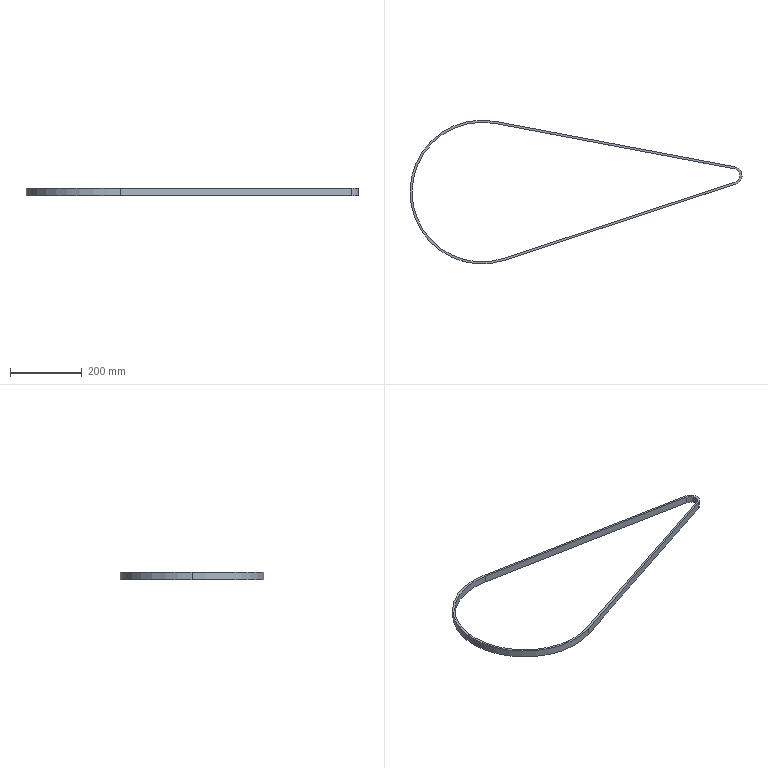Part | SolidWorks | features Sweep 1 | 1 solid | 12 faces | box 923.5 x 400 x 20 mm | volume 251339 mm3 | cylinder 6 | plane 6 | commonest cylinder face diameters 388.216 x2 400 x2 38.274 x1 50 x1
STEP:
#1=CARTESIAN_POINT('',(-778.071,-459.045,10.));
#2=VERTEX_POINT('',#1);
#3=CARTESIAN_POINT('',(-1040.663,-269.092,10.));
#4=VERTEX_POINT('',#3);
#5=CARTESIAN_POINT('',(-840.663,-269.092,10.));
#6=DIRECTION('',(0.,0.,-1.));
#7=DIRECTION('',(-1.,0.,0.));
#8=AXIS2_PLACEMENT_3D('',#5,#6,#7);
#9=CIRCLE('',#8,200.);
#10=EDGE_CURVE('',#2,#4,#9,.T.);
#11=ORIENTED_EDGE('',*,*,#10,.T.);
#12=CARTESIAN_POINT('',(-1040.663,-269.092,-10.));
#13=VERTEX_POINT('',#12);
#14=CARTESIAN_POINT('',(-1040.663,-269.092,0.));
#15=DIRECTION('',(0.,0.,-1.));
#16=VECTOR('',#15,1000.);
#17=LINE('',#14,#16);
#18=EDGE_CURVE('',#4,#13,#17,.T.);
#19=ORIENTED_EDGE('',*,*,#18,.T.);
#20=CARTESIAN_POINT('',(-778.071,-459.045,-10.));
#21=VERTEX_POINT('',#20);
#22=CARTESIAN_POINT('',(-840.663,-269.092,-10.));
#23=DIRECTION('',(0.,0.,-1.));
#24=DIRECTION('',(-1.,0.,0.));
#25=AXIS2_PLACEMENT_3D('',#22,#23,#24);
#26=CIRCLE('',#25,200.);
#27=EDGE_CURVE('',#21,#13,#26,.T.);
#28=ORIENTED_EDGE('',*,*,#27,.F.);
#29=CARTESIAN_POINT('',(-778.071,-459.045,10.));
#30=DIRECTION('',(0.,0.,1.));
#31=VECTOR('',#30,1000.);
#32=LINE('',#29,#31);
#33=EDGE_CURVE('',#21,#2,#32,.T.);
#34=ORIENTED_EDGE('',*,*,#33,.T.);
#35=EDGE_LOOP('',(#11,#19,#28,#34));
#36=FACE_OUTER_BOUND('',#35,.T.);
#37=CARTESIAN_POINT('',(-840.663,-269.092,0.));
#38=DIRECTION('',(0.,0.,-1.));
#39=DIRECTION('',(-1.,0.,0.));
#40=AXIS2_PLACEMENT_3D('',#37,#38,#39);
#41=CYLINDRICAL_SURFACE('',#40,200.);
#42=ADVANCED_FACE('',(#36),#41,.T.);
#43=CARTESIAN_POINT('',(-1034.771,-269.092,10.));
#44=VERTEX_POINT('',#43);
#45=CARTESIAN_POINT('',(-803.472,-78.58,10.));
#46=VERTEX_POINT('',#45);
#47=CARTESIAN_POINT('',(-840.663,-269.092,10.));
#48=DIRECTION('',(0.,0.,-1.));
#49=DIRECTION('',(-1.,0.,0.));
#50=AXIS2_PLACEMENT_3D('',#47,#48,#49);
#51=CIRCLE('',#50,194.108);
#52=EDGE_CURVE('',#44,#46,#51,.T.);
#53=ORIENTED_EDGE('',*,*,#52,.F.);
#54=CARTESIAN_POINT('',(-1034.771,-269.092,-10.));
#55=VERTEX_POINT('',#54);
#56=CARTESIAN_POINT('',(-1034.771,-269.092,0.));
#57=DIRECTION('',(0.,0.,-1.));
#58=VECTOR('',#57,1000.);
#59=LINE('',#56,#58);
#60=EDGE_CURVE('',#44,#55,#59,.T.);
#61=ORIENTED_EDGE('',*,*,#60,.T.);
#62=CARTESIAN_POINT('',(-803.472,-78.58,-10.));
#63=VERTEX_POINT('',#62);
#64=CARTESIAN_POINT('',(-840.663,-269.092,-10.));
#65=DIRECTION('',(0.,0.,-1.));
#66=DIRECTION('',(-1.,0.,0.));
#67=AXIS2_PLACEMENT_3D('',#64,#65,#66);
#68=CIRCLE('',#67,194.108);
#69=EDGE_CURVE('',#55,#63,#68,.T.);
#70=ORIENTED_EDGE('',*,*,#69,.T.);
#71=CARTESIAN_POINT('',(-803.472,-78.58,10.));
#72=CARTESIAN_POINT('',(-803.472,-78.58,3.333));
#73=CARTESIAN_POINT('',(-803.472,-78.58,-3.333));
#74=CARTESIAN_POINT('',(-803.472,-78.58,-10.));
#75=B_SPLINE_CURVE_WITH_KNOTS('',3,(#71,#72,#73,#74),.UNSPECIFIED.,.F.,.F.,(4,4),(0.,1.),.UNSPECIFIED.);
#76=EDGE_CURVE('',#46,#63,#75,.T.);
#77=ORIENTED_EDGE('',*,*,#76,.F.);
#78=EDGE_LOOP('',(#53,#61,#70,#77));
#79=FACE_OUTER_BOUND('',#78,.T.);
#80=CARTESIAN_POINT('',(-840.663,-269.092,0.));
#81=DIRECTION('',(0.,0.,-1.));
#82=DIRECTION('',(-1.,0.,0.));
#83=AXIS2_PLACEMENT_3D('',#80,#81,#82);
#84=CYLINDRICAL_SURFACE('',#83,194.108);
#85=ADVANCED_FACE('',(#79),#84,.F.);
#86=ORIENTED_EDGE('',*,*,#60,.F.);
#87=CARTESIAN_POINT('',(-780.976,-453.795,10.));
#88=VERTEX_POINT('',#87);
#89=CARTESIAN_POINT('',(-840.663,-269.092,10.));
#90=DIRECTION('',(0.,0.,-1.));
#91=DIRECTION('',(-1.,0.,0.));
#92=AXIS2_PLACEMENT_3D('',#89,#90,#91);
#93=CIRCLE('',#92,194.108);
#94=EDGE_CURVE('',#88,#44,#93,.T.);
#95=ORIENTED_EDGE('',*,*,#94,.F.);
#96=CARTESIAN_POINT('',(-780.976,-453.795,-10.));
#97=VERTEX_POINT('',#96);
#98=CARTESIAN_POINT('',(-780.976,-453.795,10.));
#99=DIRECTION('',(0.,0.,-1.));
#100=VECTOR('',#99,1000.);
#101=LINE('',#98,#100);
#102=EDGE_CURVE('',#88,#97,#101,.T.);
#103=ORIENTED_EDGE('',*,*,#102,.T.);
#104=CARTESIAN_POINT('',(-840.663,-269.092,-10.));
#105=DIRECTION('',(0.,0.,-1.));
#106=DIRECTION('',(-1.,0.,0.));
#107=AXIS2_PLACEMENT_3D('',#104,#105,#106);
#108=CIRCLE('',#107,194.108);
#109=EDGE_CURVE('',#97,#55,#108,.T.);
#110=ORIENTED_EDGE('',*,*,#109,.T.);
#111=EDGE_LOOP('',(#86,#95,#103,#110));
#112=FACE_OUTER_BOUND('',#111,.T.);
#113=CARTESIAN_POINT('',(-840.663,-269.092,0.));
#114=DIRECTION('',(0.,0.,-1.));
#115=DIRECTION('',(-1.,0.,0.));
#116=AXIS2_PLACEMENT_3D('',#113,#114,#115);
#117=CYLINDRICAL_SURFACE('',#116,194.108);
#118=ADVANCED_FACE('',(#112),#117,.F.);
#119=ORIENTED_EDGE('',*,*,#18,.F.);
#120=CARTESIAN_POINT('',(-803.472,-72.58,10.));
#121=VERTEX_POINT('',#120);
#122=CARTESIAN_POINT('',(-840.663,-269.092,10.));
#123=DIRECTION('',(0.,0.,-1.));
#124=DIRECTION('',(-1.,0.,0.));
#125=AXIS2_PLACEMENT_3D('',#122,#123,#124);
#126=CIRCLE('',#125,200.);
#127=EDGE_CURVE('',#4,#121,#126,.T.);
#128=ORIENTED_EDGE('',*,*,#127,.T.);
#129=CARTESIAN_POINT('',(-803.472,-72.58,-10.));
#130=VERTEX_POINT('',#129);
#131=CARTESIAN_POINT('',(-803.472,-72.58,-10.));
#132=CARTESIAN_POINT('',(-803.472,-72.58,-3.333));
#133=CARTESIAN_POINT('',(-803.472,-72.58,3.333));
#134=CARTESIAN_POINT('',(-803.472,-72.58,10.));
#135=B_SPLINE_CURVE_WITH_KNOTS('',3,(#131,#132,#133,#134),.UNSPECIFIED.,.F.,.F.,(4,4),(0.,1.),.UNSPECIFIED.);
#136=EDGE_CURVE('',#130,#121,#135,.T.);
#137=ORIENTED_EDGE('',*,*,#136,.F.);
#138=CARTESIAN_POINT('',(-840.663,-269.092,-10.));
#139=DIRECTION('',(0.,0.,-1.));
#140=DIRECTION('',(-1.,0.,0.));
#141=AXIS2_PLACEMENT_3D('',#138,#139,#140);
#142=CIRCLE('',#141,200.);
#143=EDGE_CURVE('',#13,#130,#142,.T.);
#144=ORIENTED_EDGE('',*,*,#143,.F.);
#145=EDGE_LOOP('',(#119,#128,#137,#144));
#146=FACE_OUTER_BOUND('',#145,.T.);
#147=CARTESIAN_POINT('',(-840.663,-269.092,0.));
#148=DIRECTION('',(0.,0.,-1.));
#149=DIRECTION('',(-1.,0.,0.));
#150=AXIS2_PLACEMENT_3D('',#147,#148,#149);
#151=CYLINDRICAL_SURFACE('',#150,200.);
#152=ADVANCED_FACE('',(#146),#151,.T.);
#153=CARTESIAN_POINT('',(-137.244,-241.677,10.));
#154=VERTEX_POINT('',#153);
#155=CARTESIAN_POINT('',(-137.244,-241.677,-10.));
#156=VERTEX_POINT('',#155);
#157=CARTESIAN_POINT('',(-137.244,-241.677,10.));
#158=DIRECTION('',(0.,0.,-1.));
#159=VECTOR('',#158,1000.);
#160=LINE('',#157,#159);
#161=EDGE_CURVE('',#154,#156,#160,.T.);
#162=ORIENTED_EDGE('',*,*,#161,.T.);
#163=CARTESIAN_POINT('',(-137.244,-241.677,-10.));
#164=DIRECTION('',(-0.9498,-0.313,0.));
#165=VECTOR('',#164,1000.);
#166=LINE('',#163,#165);
#167=EDGE_CURVE('',#156,#97,#166,.T.);
#168=ORIENTED_EDGE('',*,*,#167,.T.);
#169=ORIENTED_EDGE('',*,*,#102,.F.);
#170=CARTESIAN_POINT('',(-137.244,-241.677,10.));
#171=DIRECTION('',(-0.9498,-0.313,0.));
#172=VECTOR('',#171,1000.);
#173=LINE('',#170,#172);
#174=EDGE_CURVE('',#154,#88,#173,.T.);
#175=ORIENTED_EDGE('',*,*,#174,.F.);
#176=EDGE_LOOP('',(#162,#168,#169,#175));
#177=FACE_OUTER_BOUND('',#176,.T.);
#178=CARTESIAN_POINT('',(-137.244,-241.677,10.));
#179=DIRECTION('',(-0.313,0.9498,0.));
#180=DIRECTION('',(-0.9498,-0.313,0.));
#181=AXIS2_PLACEMENT_3D('',#178,#179,#180);
#182=PLANE('',#181);
#183=ADVANCED_FACE('',(#177),#182,.T.);
#184=CARTESIAN_POINT('',(-134.34,-246.927,-10.));
#185=VERTEX_POINT('',#184);
#186=CARTESIAN_POINT('',(-134.34,-246.927,10.));
#187=VERTEX_POINT('',#186);
#188=CARTESIAN_POINT('',(-134.34,-246.927,10.));
#189=DIRECTION('',(0.,0.,1.));
#190=VECTOR('',#189,1000.);
#191=LINE('',#188,#190);
#192=EDGE_CURVE('',#185,#187,#191,.T.);
#193=ORIENTED_EDGE('',*,*,#192,.T.);
#194=CARTESIAN_POINT('',(-134.34,-246.927,10.));
#195=DIRECTION('',(-0.9498,-0.313,0.));
#196=VECTOR('',#195,1000.);
#197=LINE('',#194,#196);
#198=EDGE_CURVE('',#187,#2,#197,.T.);
#199=ORIENTED_EDGE('',*,*,#198,.T.);
#200=ORIENTED_EDGE('',*,*,#33,.F.);
#201=CARTESIAN_POINT('',(-134.34,-246.927,-10.));
#202=DIRECTION('',(-0.9498,-0.313,0.));
#203=VECTOR('',#202,1000.);
#204=LINE('',#201,#203);
#205=EDGE_CURVE('',#185,#21,#204,.T.);
#206=ORIENTED_EDGE('',*,*,#205,.F.);
#207=EDGE_LOOP('',(#193,#199,#200,#206));
#208=FACE_OUTER_BOUND('',#207,.T.);
#209=CARTESIAN_POINT('',(-134.34,-246.927,10.));
#210=DIRECTION('',(0.313,-0.9498,0.));
#211=DIRECTION('',(0.9498,0.313,0.));
#212=AXIS2_PLACEMENT_3D('',#209,#210,#211);
#213=PLANE('',#212);
#214=ADVANCED_FACE('',(#208),#213,.T.);
#215=CARTESIAN_POINT('',(-137.515,-204.619,10.));
#216=VERTEX_POINT('',#215);
#217=CARTESIAN_POINT('',(-137.515,-204.619,-10.));
#218=VERTEX_POINT('',#217);
#219=CARTESIAN_POINT('',(-137.515,-204.619,10.));
#220=DIRECTION('',(0.,0.,-1.));
#221=VECTOR('',#220,1000.);
#222=LINE('',#219,#221);
#223=EDGE_CURVE('',#216,#218,#222,.T.);
#224=ORIENTED_EDGE('',*,*,#223,.T.);
#225=CARTESIAN_POINT('',(-142.164,-223.183,-10.));
#226=DIRECTION('',(0.,0.,-1.));
#227=DIRECTION('',(-1.,0.,0.));
#228=AXIS2_PLACEMENT_3D('',#225,#226,#227);
#229=CIRCLE('',#228,19.137);
#230=EDGE_CURVE('',#218,#156,#229,.T.);
#231=ORIENTED_EDGE('',*,*,#230,.T.);
#232=ORIENTED_EDGE('',*,*,#161,.F.);
#233=CARTESIAN_POINT('',(-142.164,-223.183,10.));
#234=DIRECTION('',(0.,0.,-1.));
#235=DIRECTION('',(-1.,0.,0.));
#236=AXIS2_PLACEMENT_3D('',#233,#234,#235);
#237=CIRCLE('',#236,19.137);
#238=EDGE_CURVE('',#216,#154,#237,.T.);
#239=ORIENTED_EDGE('',*,*,#238,.F.);
#240=EDGE_LOOP('',(#224,#231,#232,#239));
#241=FACE_OUTER_BOUND('',#240,.T.);
#242=CARTESIAN_POINT('',(-142.164,-223.183,0.));
#243=DIRECTION('',(0.,0.,-1.));
#244=DIRECTION('',(-1.,0.,0.));
#245=AXIS2_PLACEMENT_3D('',#242,#243,#244);
#246=CYLINDRICAL_SURFACE('',#245,19.137);
#247=ADVANCED_FACE('',(#241),#246,.F.);
#248=CARTESIAN_POINT('',(-137.515,-198.619,-10.));
#249=VERTEX_POINT('',#248);
#250=CARTESIAN_POINT('',(-137.515,-198.619,10.));
#251=VERTEX_POINT('',#250);
#252=CARTESIAN_POINT('',(-137.515,-198.619,10.));
#253=DIRECTION('',(0.,0.,1.));
#254=VECTOR('',#253,1000.);
#255=LINE('',#252,#254);
#256=EDGE_CURVE('',#249,#251,#255,.T.);
#257=ORIENTED_EDGE('',*,*,#256,.T.);
#258=CARTESIAN_POINT('',(-142.164,-223.183,10.));
#259=DIRECTION('',(0.,0.,-1.));
#260=DIRECTION('',(-1.,0.,0.));
#261=AXIS2_PLACEMENT_3D('',#258,#259,#260);
#262=CIRCLE('',#261,25.);
#263=EDGE_CURVE('',#251,#187,#262,.T.);
#264=ORIENTED_EDGE('',*,*,#263,.T.);
#265=ORIENTED_EDGE('',*,*,#192,.F.);
#266=CARTESIAN_POINT('',(-142.164,-223.183,-10.));
#267=DIRECTION('',(0.,0.,-1.));
#268=DIRECTION('',(-1.,0.,0.));
#269=AXIS2_PLACEMENT_3D('',#266,#267,#268);
#270=CIRCLE('',#269,25.);
#271=EDGE_CURVE('',#249,#185,#270,.T.);
#272=ORIENTED_EDGE('',*,*,#271,.F.);
#273=EDGE_LOOP('',(#257,#264,#265,#272));
#274=FACE_OUTER_BOUND('',#273,.T.);
#275=CARTESIAN_POINT('',(-142.164,-223.183,0.));
#276=DIRECTION('',(0.,0.,-1.));
#277=DIRECTION('',(-1.,0.,0.));
#278=AXIS2_PLACEMENT_3D('',#275,#276,#277);
#279=CYLINDRICAL_SURFACE('',#278,25.);
#280=ADVANCED_FACE('',(#274),#279,.T.);
#281=CARTESIAN_POINT('',(-137.515,-204.619,10.));
#282=DIRECTION('',(-0.9826,0.186,0.));
#283=VECTOR('',#282,1000.);
#284=LINE('',#281,#283);
#285=EDGE_CURVE('',#216,#46,#284,.T.);
#286=ORIENTED_EDGE('',*,*,#285,.F.);
#287=ORIENTED_EDGE('',*,*,#238,.T.);
#288=ORIENTED_EDGE('',*,*,#174,.T.);
#289=ORIENTED_EDGE('',*,*,#94,.T.);
#290=ORIENTED_EDGE('',*,*,#52,.T.);
#291=EDGE_LOOP('',(#286,#287,#288,#289,#290));
#292=FACE_BOUND('',#291,.T.);
#293=CARTESIAN_POINT('',(-137.515,-198.619,10.));
#294=DIRECTION('',(-0.9826,0.186,0.));
#295=VECTOR('',#294,1000.);
#296=LINE('',#293,#295);
#297=EDGE_CURVE('',#251,#121,#296,.T.);
#298=ORIENTED_EDGE('',*,*,#297,.T.);
#299=ORIENTED_EDGE('',*,*,#127,.F.);
#300=ORIENTED_EDGE('',*,*,#10,.F.);
#301=ORIENTED_EDGE('',*,*,#198,.F.);
#302=ORIENTED_EDGE('',*,*,#263,.F.);
#303=EDGE_LOOP('',(#298,#299,#300,#301,#302));
#304=FACE_OUTER_BOUND('',#303,.T.);
#305=CARTESIAN_POINT('',(-137.515,-198.619,10.));
#306=DIRECTION('',(0.,0.,-1.));
#307=DIRECTION('',(0.,1.,0.));
#308=AXIS2_PLACEMENT_3D('',#305,#306,#307);
#309=PLANE('',#308);
#310=ADVANCED_FACE('',(#292,#304),#309,.F.);
#311=ORIENTED_EDGE('',*,*,#76,.T.);
#312=CARTESIAN_POINT('',(-137.515,-204.619,-10.));
#313=DIRECTION('',(-0.9826,0.186,0.));
#314=VECTOR('',#313,1000.);
#315=LINE('',#312,#314);
#316=EDGE_CURVE('',#218,#63,#315,.T.);
#317=ORIENTED_EDGE('',*,*,#316,.F.);
#318=ORIENTED_EDGE('',*,*,#223,.F.);
#319=ORIENTED_EDGE('',*,*,#285,.T.);
#320=EDGE_LOOP('',(#311,#317,#318,#319));
#321=FACE_OUTER_BOUND('',#320,.T.);
#322=CARTESIAN_POINT('',(-137.515,-204.619,10.));
#323=DIRECTION('',(0.186,0.9826,0.));
#324=DIRECTION('',(-0.9826,0.186,0.));
#325=AXIS2_PLACEMENT_3D('',#322,#323,#324);
#326=PLANE('',#325);
#327=ADVANCED_FACE('',(#321),#326,.F.);
#328=CARTESIAN_POINT('',(-137.515,-198.619,-10.));
#329=DIRECTION('',(-0.9826,0.186,0.));
#330=VECTOR('',#329,1000.);
#331=LINE('',#328,#330);
#332=EDGE_CURVE('',#249,#130,#331,.T.);
#333=ORIENTED_EDGE('',*,*,#332,.F.);
#334=ORIENTED_EDGE('',*,*,#271,.T.);
#335=ORIENTED_EDGE('',*,*,#205,.T.);
#336=ORIENTED_EDGE('',*,*,#27,.T.);
#337=ORIENTED_EDGE('',*,*,#143,.T.);
#338=EDGE_LOOP('',(#333,#334,#335,#336,#337));
#339=FACE_OUTER_BOUND('',#338,.T.);
#340=ORIENTED_EDGE('',*,*,#316,.T.);
#341=ORIENTED_EDGE('',*,*,#69,.F.);
#342=ORIENTED_EDGE('',*,*,#109,.F.);
#343=ORIENTED_EDGE('',*,*,#167,.F.);
#344=ORIENTED_EDGE('',*,*,#230,.F.);
#345=EDGE_LOOP('',(#340,#341,#342,#343,#344));
#346=FACE_BOUND('',#345,.T.);
#347=CARTESIAN_POINT('',(-137.515,-198.619,-10.));
#348=DIRECTION('',(0.,0.,1.));
#349=DIRECTION('',(1.,0.,0.));
#350=AXIS2_PLACEMENT_3D('',#347,#348,#349);
#351=PLANE('',#350);
#352=ADVANCED_FACE('',(#339,#346),#351,.F.);
#353=ORIENTED_EDGE('',*,*,#136,.T.);
#354=ORIENTED_EDGE('',*,*,#297,.F.);
#355=ORIENTED_EDGE('',*,*,#256,.F.);
#356=ORIENTED_EDGE('',*,*,#332,.T.);
#357=EDGE_LOOP('',(#353,#354,#355,#356));
#358=FACE_OUTER_BOUND('',#357,.T.);
#359=CARTESIAN_POINT('',(-137.515,-198.619,10.));
#360=DIRECTION('',(-0.186,-0.9826,0.));
#361=DIRECTION('',(0.9826,-0.186,0.));
#362=AXIS2_PLACEMENT_3D('',#359,#360,#361);
#363=PLANE('',#362);
#364=ADVANCED_FACE('',(#358),#363,.F.);
#365=CLOSED_SHELL('',(#42,#85,#118,#152,#183,#214,#247,#280,#310,#327,#352,#364));
#366=MANIFOLD_SOLID_BREP('',#365);
#367=CARTESIAN_POINT('',(0.,0.,0.));
#368=DIRECTION('',(0.,0.,1.));
#369=DIRECTION('',(1.,0.,0.));
#370=AXIS2_PLACEMENT_3D('',#367,#368,#369);
#371=(LENGTH_UNIT()NAMED_UNIT(*)SI_UNIT(.MILLI.,.METRE.));
#372=UNCERTAINTY_MEASURE_WITH_UNIT(LENGTH_MEASURE(0.00001),#371,'','');
#373=(NAMED_UNIT(*)PLANE_ANGLE_UNIT()SI_UNIT($,.RADIAN.));
#374=(NAMED_UNIT(*)SI_UNIT($,.STERADIAN.)SOLID_ANGLE_UNIT());
#375=(GEOMETRIC_REPRESENTATION_CONTEXT(3)GLOBAL_UNCERTAINTY_ASSIGNED_CONTEXT((#372))GLOBAL_UNIT_ASSIGNED_CONTEXT((#371,#373,#374))REPRESENTATION_CONTEXT('',''));
#376=ADVANCED_BREP_SHAPE_REPRESENTATION('',(#366,#370),#375);